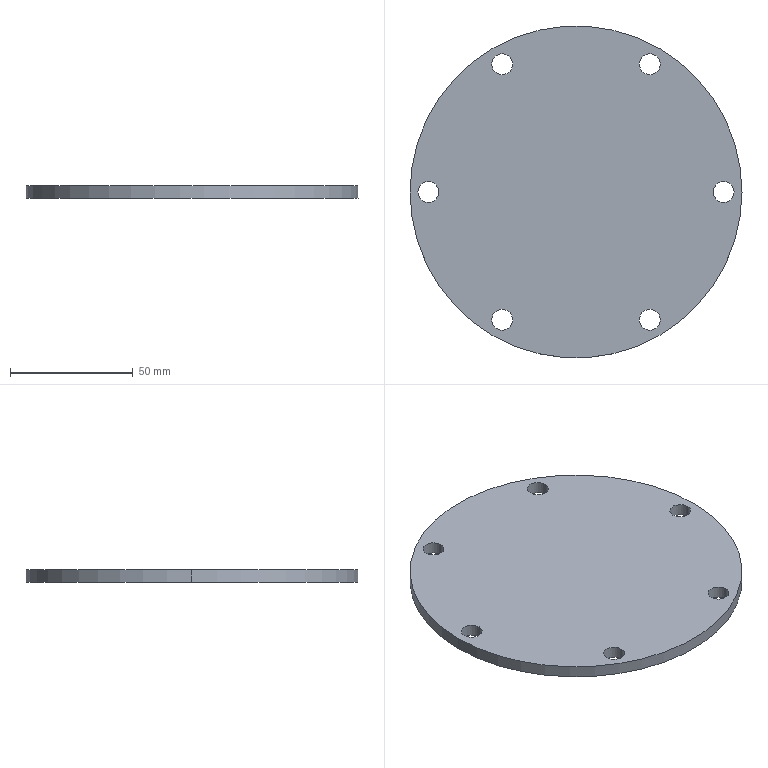Part | SolidWorks | features CirPattern 1, FlatPattern 1, ICE 1, SMBaseFlange 1, SheetMetal 1 | 1 solid | 16 faces | box 135 x 135 x 5 mm | volume 69867 mm3 | cylinder 14 | plane 2 | commonest cylinder face diameters 8.5 x12 135 x2
STEP:
#1=CARTESIAN_POINT('',(25.75,51.962,-5.));
#2=VERTEX_POINT('',#1);
#3=CARTESIAN_POINT('',(34.25,51.962,-5.));
#4=VERTEX_POINT('',#3);
#5=CARTESIAN_POINT('',(30.,51.962,-5.));
#6=DIRECTION('',(0.,0.,1.));
#7=DIRECTION('',(1.,0.,0.));
#8=AXIS2_PLACEMENT_3D('',#5,#6,#7);
#9=CIRCLE('',#8,4.25);
#10=EDGE_CURVE('',#2,#4,#9,.T.);
#11=ORIENTED_EDGE('',*,*,#10,.F.);
#12=CARTESIAN_POINT('',(25.75,51.962,0.));
#13=VERTEX_POINT('',#12);
#14=CARTESIAN_POINT('',(25.75,51.962,-10.));
#15=DIRECTION('',(0.,0.,1.));
#16=VECTOR('',#15,1000.);
#17=LINE('',#14,#16);
#18=EDGE_CURVE('',#2,#13,#17,.T.);
#19=ORIENTED_EDGE('',*,*,#18,.T.);
#20=CARTESIAN_POINT('',(34.25,51.962,0.));
#21=VERTEX_POINT('',#20);
#22=CARTESIAN_POINT('',(30.,51.962,0.));
#23=DIRECTION('',(0.,0.,1.));
#24=DIRECTION('',(0.5,0.866,0.));
#25=AXIS2_PLACEMENT_3D('',#22,#23,#24);
#26=CIRCLE('',#25,4.25);
#27=EDGE_CURVE('',#13,#21,#26,.T.);
#28=ORIENTED_EDGE('',*,*,#27,.T.);
#29=CARTESIAN_POINT('',(34.25,51.962,-10.));
#30=DIRECTION('',(0.,0.,1.));
#31=VECTOR('',#30,1000.);
#32=LINE('',#29,#31);
#33=EDGE_CURVE('',#4,#21,#32,.T.);
#34=ORIENTED_EDGE('',*,*,#33,.F.);
#35=EDGE_LOOP('',(#11,#19,#28,#34));
#36=FACE_OUTER_BOUND('',#35,.T.);
#37=CARTESIAN_POINT('',(30.,51.962,-10.));
#38=DIRECTION('',(0.,0.,1.));
#39=DIRECTION('',(1.,0.,0.));
#40=AXIS2_PLACEMENT_3D('',#37,#38,#39);
#41=CYLINDRICAL_SURFACE('',#40,4.25);
#42=ADVANCED_FACE('',(#36),#41,.F.);
#43=CARTESIAN_POINT('',(-34.25,51.962,-5.));
#44=VERTEX_POINT('',#43);
#45=CARTESIAN_POINT('',(-25.75,51.962,-5.));
#46=VERTEX_POINT('',#45);
#47=CARTESIAN_POINT('',(-30.,51.962,-5.));
#48=DIRECTION('',(0.,0.,1.));
#49=DIRECTION('',(1.,0.,0.));
#50=AXIS2_PLACEMENT_3D('',#47,#48,#49);
#51=CIRCLE('',#50,4.25);
#52=EDGE_CURVE('',#44,#46,#51,.T.);
#53=ORIENTED_EDGE('',*,*,#52,.F.);
#54=CARTESIAN_POINT('',(-34.25,51.962,0.));
#55=VERTEX_POINT('',#54);
#56=CARTESIAN_POINT('',(-34.25,51.962,-10.));
#57=DIRECTION('',(0.,0.,1.));
#58=VECTOR('',#57,1000.);
#59=LINE('',#56,#58);
#60=EDGE_CURVE('',#44,#55,#59,.T.);
#61=ORIENTED_EDGE('',*,*,#60,.T.);
#62=CARTESIAN_POINT('',(-25.75,51.962,0.));
#63=VERTEX_POINT('',#62);
#64=CARTESIAN_POINT('',(-30.,51.962,0.));
#65=DIRECTION('',(0.,0.,1.));
#66=DIRECTION('',(-0.5,0.866,0.));
#67=AXIS2_PLACEMENT_3D('',#64,#65,#66);
#68=CIRCLE('',#67,4.25);
#69=EDGE_CURVE('',#55,#63,#68,.T.);
#70=ORIENTED_EDGE('',*,*,#69,.T.);
#71=CARTESIAN_POINT('',(-25.75,51.962,-10.));
#72=DIRECTION('',(0.,0.,1.));
#73=VECTOR('',#72,1000.);
#74=LINE('',#71,#73);
#75=EDGE_CURVE('',#46,#63,#74,.T.);
#76=ORIENTED_EDGE('',*,*,#75,.F.);
#77=EDGE_LOOP('',(#53,#61,#70,#76));
#78=FACE_OUTER_BOUND('',#77,.T.);
#79=CARTESIAN_POINT('',(-30.,51.962,-10.));
#80=DIRECTION('',(0.,0.,1.));
#81=DIRECTION('',(1.,0.,0.));
#82=AXIS2_PLACEMENT_3D('',#79,#80,#81);
#83=CYLINDRICAL_SURFACE('',#82,4.25);
#84=ADVANCED_FACE('',(#78),#83,.F.);
#85=CARTESIAN_POINT('',(-64.25,0.,-5.));
#86=VERTEX_POINT('',#85);
#87=CARTESIAN_POINT('',(-55.75,0.,-5.));
#88=VERTEX_POINT('',#87);
#89=CARTESIAN_POINT('',(-60.,0.,-5.));
#90=DIRECTION('',(0.,0.,1.));
#91=DIRECTION('',(1.,0.,0.));
#92=AXIS2_PLACEMENT_3D('',#89,#90,#91);
#93=CIRCLE('',#92,4.25);
#94=EDGE_CURVE('',#86,#88,#93,.T.);
#95=ORIENTED_EDGE('',*,*,#94,.F.);
#96=CARTESIAN_POINT('',(-64.25,0.,0.));
#97=VERTEX_POINT('',#96);
#98=CARTESIAN_POINT('',(-64.25,0.,-10.));
#99=DIRECTION('',(0.,0.,1.));
#100=VECTOR('',#99,1000.);
#101=LINE('',#98,#100);
#102=EDGE_CURVE('',#86,#97,#101,.T.);
#103=ORIENTED_EDGE('',*,*,#102,.T.);
#104=CARTESIAN_POINT('',(-55.75,0.,0.));
#105=VERTEX_POINT('',#104);
#106=CARTESIAN_POINT('',(-60.,0.,0.));
#107=DIRECTION('',(0.,0.,1.));
#108=DIRECTION('',(-1.,0.,0.));
#109=AXIS2_PLACEMENT_3D('',#106,#107,#108);
#110=CIRCLE('',#109,4.25);
#111=EDGE_CURVE('',#97,#105,#110,.T.);
#112=ORIENTED_EDGE('',*,*,#111,.T.);
#113=CARTESIAN_POINT('',(-55.75,0.,-10.));
#114=DIRECTION('',(0.,0.,1.));
#115=VECTOR('',#114,1000.);
#116=LINE('',#113,#115);
#117=EDGE_CURVE('',#88,#105,#116,.T.);
#118=ORIENTED_EDGE('',*,*,#117,.F.);
#119=EDGE_LOOP('',(#95,#103,#112,#118));
#120=FACE_OUTER_BOUND('',#119,.T.);
#121=CARTESIAN_POINT('',(-60.,0.,-10.));
#122=DIRECTION('',(0.,0.,1.));
#123=DIRECTION('',(1.,0.,0.));
#124=AXIS2_PLACEMENT_3D('',#121,#122,#123);
#125=CYLINDRICAL_SURFACE('',#124,4.25);
#126=ADVANCED_FACE('',(#120),#125,.F.);
#127=CARTESIAN_POINT('',(-34.25,-51.962,-5.));
#128=VERTEX_POINT('',#127);
#129=CARTESIAN_POINT('',(-25.75,-51.962,-5.));
#130=VERTEX_POINT('',#129);
#131=CARTESIAN_POINT('',(-30.,-51.962,-5.));
#132=DIRECTION('',(0.,0.,1.));
#133=DIRECTION('',(1.,0.,0.));
#134=AXIS2_PLACEMENT_3D('',#131,#132,#133);
#135=CIRCLE('',#134,4.25);
#136=EDGE_CURVE('',#128,#130,#135,.T.);
#137=ORIENTED_EDGE('',*,*,#136,.F.);
#138=CARTESIAN_POINT('',(-34.25,-51.962,0.));
#139=VERTEX_POINT('',#138);
#140=CARTESIAN_POINT('',(-34.25,-51.962,-10.));
#141=DIRECTION('',(0.,0.,1.));
#142=VECTOR('',#141,1000.);
#143=LINE('',#140,#142);
#144=EDGE_CURVE('',#128,#139,#143,.T.);
#145=ORIENTED_EDGE('',*,*,#144,.T.);
#146=CARTESIAN_POINT('',(-25.75,-51.962,0.));
#147=VERTEX_POINT('',#146);
#148=CARTESIAN_POINT('',(-30.,-51.962,0.));
#149=DIRECTION('',(0.,0.,1.));
#150=DIRECTION('',(-0.5,-0.866,0.));
#151=AXIS2_PLACEMENT_3D('',#148,#149,#150);
#152=CIRCLE('',#151,4.25);
#153=EDGE_CURVE('',#139,#147,#152,.T.);
#154=ORIENTED_EDGE('',*,*,#153,.T.);
#155=CARTESIAN_POINT('',(-25.75,-51.962,-10.));
#156=DIRECTION('',(0.,0.,1.));
#157=VECTOR('',#156,1000.);
#158=LINE('',#155,#157);
#159=EDGE_CURVE('',#130,#147,#158,.T.);
#160=ORIENTED_EDGE('',*,*,#159,.F.);
#161=EDGE_LOOP('',(#137,#145,#154,#160));
#162=FACE_OUTER_BOUND('',#161,.T.);
#163=CARTESIAN_POINT('',(-30.,-51.962,-10.));
#164=DIRECTION('',(0.,0.,1.));
#165=DIRECTION('',(1.,0.,0.));
#166=AXIS2_PLACEMENT_3D('',#163,#164,#165);
#167=CYLINDRICAL_SURFACE('',#166,4.25);
#168=ADVANCED_FACE('',(#162),#167,.F.);
#169=CARTESIAN_POINT('',(25.75,-51.962,-5.));
#170=VERTEX_POINT('',#169);
#171=CARTESIAN_POINT('',(34.25,-51.962,-5.));
#172=VERTEX_POINT('',#171);
#173=CARTESIAN_POINT('',(30.,-51.962,-5.));
#174=DIRECTION('',(0.,0.,1.));
#175=DIRECTION('',(1.,0.,0.));
#176=AXIS2_PLACEMENT_3D('',#173,#174,#175);
#177=CIRCLE('',#176,4.25);
#178=EDGE_CURVE('',#170,#172,#177,.T.);
#179=ORIENTED_EDGE('',*,*,#178,.F.);
#180=CARTESIAN_POINT('',(25.75,-51.962,0.));
#181=VERTEX_POINT('',#180);
#182=CARTESIAN_POINT('',(25.75,-51.962,-10.));
#183=DIRECTION('',(0.,0.,1.));
#184=VECTOR('',#183,1000.);
#185=LINE('',#182,#184);
#186=EDGE_CURVE('',#170,#181,#185,.T.);
#187=ORIENTED_EDGE('',*,*,#186,.T.);
#188=CARTESIAN_POINT('',(34.25,-51.962,0.));
#189=VERTEX_POINT('',#188);
#190=CARTESIAN_POINT('',(30.,-51.962,0.));
#191=DIRECTION('',(0.,0.,1.));
#192=DIRECTION('',(0.5,-0.866,0.));
#193=AXIS2_PLACEMENT_3D('',#190,#191,#192);
#194=CIRCLE('',#193,4.25);
#195=EDGE_CURVE('',#181,#189,#194,.T.);
#196=ORIENTED_EDGE('',*,*,#195,.T.);
#197=CARTESIAN_POINT('',(34.25,-51.962,-10.));
#198=DIRECTION('',(0.,0.,1.));
#199=VECTOR('',#198,1000.);
#200=LINE('',#197,#199);
#201=EDGE_CURVE('',#172,#189,#200,.T.);
#202=ORIENTED_EDGE('',*,*,#201,.F.);
#203=EDGE_LOOP('',(#179,#187,#196,#202));
#204=FACE_OUTER_BOUND('',#203,.T.);
#205=CARTESIAN_POINT('',(30.,-51.962,-10.));
#206=DIRECTION('',(0.,0.,1.));
#207=DIRECTION('',(1.,0.,0.));
#208=AXIS2_PLACEMENT_3D('',#205,#206,#207);
#209=CYLINDRICAL_SURFACE('',#208,4.25);
#210=ADVANCED_FACE('',(#204),#209,.F.);
#211=CARTESIAN_POINT('',(55.75,0.,-5.));
#212=VERTEX_POINT('',#211);
#213=CARTESIAN_POINT('',(64.25,0.,-5.));
#214=VERTEX_POINT('',#213);
#215=CARTESIAN_POINT('',(60.,0.,-5.));
#216=DIRECTION('',(0.,0.,1.));
#217=DIRECTION('',(1.,0.,0.));
#218=AXIS2_PLACEMENT_3D('',#215,#216,#217);
#219=CIRCLE('',#218,4.25);
#220=EDGE_CURVE('',#212,#214,#219,.T.);
#221=ORIENTED_EDGE('',*,*,#220,.F.);
#222=CARTESIAN_POINT('',(55.75,0.,0.));
#223=VERTEX_POINT('',#222);
#224=CARTESIAN_POINT('',(55.75,0.,-10.));
#225=DIRECTION('',(0.,0.,1.));
#226=VECTOR('',#225,1000.);
#227=LINE('',#224,#226);
#228=EDGE_CURVE('',#212,#223,#227,.T.);
#229=ORIENTED_EDGE('',*,*,#228,.T.);
#230=CARTESIAN_POINT('',(64.25,0.,0.));
#231=VERTEX_POINT('',#230);
#232=CARTESIAN_POINT('',(60.,0.,0.));
#233=DIRECTION('',(0.,0.,1.));
#234=DIRECTION('',(1.,0.,0.));
#235=AXIS2_PLACEMENT_3D('',#232,#233,#234);
#236=CIRCLE('',#235,4.25);
#237=EDGE_CURVE('',#223,#231,#236,.T.);
#238=ORIENTED_EDGE('',*,*,#237,.T.);
#239=CARTESIAN_POINT('',(64.25,0.,-10.));
#240=DIRECTION('',(0.,0.,1.));
#241=VECTOR('',#240,1000.);
#242=LINE('',#239,#241);
#243=EDGE_CURVE('',#214,#231,#242,.T.);
#244=ORIENTED_EDGE('',*,*,#243,.F.);
#245=EDGE_LOOP('',(#221,#229,#238,#244));
#246=FACE_OUTER_BOUND('',#245,.T.);
#247=CARTESIAN_POINT('',(60.,0.,-10.));
#248=DIRECTION('',(0.,0.,1.));
#249=DIRECTION('',(1.,0.,0.));
#250=AXIS2_PLACEMENT_3D('',#247,#248,#249);
#251=CYLINDRICAL_SURFACE('',#250,4.25);
#252=ADVANCED_FACE('',(#246),#251,.F.);
#253=CARTESIAN_POINT('',(67.5,0.,-5.));
#254=VERTEX_POINT('',#253);
#255=CARTESIAN_POINT('',(-67.5,0.,-5.));
#256=VERTEX_POINT('',#255);
#257=CARTESIAN_POINT('',(0.,0.,-5.));
#258=DIRECTION('',(0.,0.,1.));
#259=DIRECTION('',(1.,0.,0.));
#260=AXIS2_PLACEMENT_3D('',#257,#258,#259);
#261=CIRCLE('',#260,67.5);
#262=EDGE_CURVE('',#254,#256,#261,.T.);
#263=ORIENTED_EDGE('',*,*,#262,.T.);
#264=CARTESIAN_POINT('',(-67.5,0.,0.));
#265=VERTEX_POINT('',#264);
#266=CARTESIAN_POINT('',(-67.5,0.,-5.));
#267=DIRECTION('',(0.,0.,1.));
#268=VECTOR('',#267,1000.);
#269=LINE('',#266,#268);
#270=EDGE_CURVE('',#256,#265,#269,.T.);
#271=ORIENTED_EDGE('',*,*,#270,.T.);
#272=CARTESIAN_POINT('',(67.5,0.,0.));
#273=VERTEX_POINT('',#272);
#274=CARTESIAN_POINT('',(0.,0.,0.));
#275=DIRECTION('',(0.,0.,1.));
#276=DIRECTION('',(1.,0.,0.));
#277=AXIS2_PLACEMENT_3D('',#274,#275,#276);
#278=CIRCLE('',#277,67.5);
#279=EDGE_CURVE('',#273,#265,#278,.T.);
#280=ORIENTED_EDGE('',*,*,#279,.F.);
#281=CARTESIAN_POINT('',(67.5,0.,-5.));
#282=DIRECTION('',(0.,0.,1.));
#283=VECTOR('',#282,1000.);
#284=LINE('',#281,#283);
#285=EDGE_CURVE('',#254,#273,#284,.T.);
#286=ORIENTED_EDGE('',*,*,#285,.F.);
#287=EDGE_LOOP('',(#263,#271,#280,#286));
#288=FACE_OUTER_BOUND('',#287,.T.);
#289=CARTESIAN_POINT('',(0.,0.,-5.));
#290=DIRECTION('',(0.,0.,1.));
#291=DIRECTION('',(1.,0.,0.));
#292=AXIS2_PLACEMENT_3D('',#289,#290,#291);
#293=CYLINDRICAL_SURFACE('',#292,67.5);
#294=ADVANCED_FACE('',(#288),#293,.T.);
#295=ORIENTED_EDGE('',*,*,#270,.F.);
#296=CARTESIAN_POINT('',(0.,0.,-5.));
#297=DIRECTION('',(0.,0.,1.));
#298=DIRECTION('',(1.,0.,0.));
#299=AXIS2_PLACEMENT_3D('',#296,#297,#298);
#300=CIRCLE('',#299,67.5);
#301=EDGE_CURVE('',#256,#254,#300,.T.);
#302=ORIENTED_EDGE('',*,*,#301,.T.);
#303=ORIENTED_EDGE('',*,*,#285,.T.);
#304=CARTESIAN_POINT('',(0.,0.,0.));
#305=DIRECTION('',(0.,0.,1.));
#306=DIRECTION('',(1.,0.,0.));
#307=AXIS2_PLACEMENT_3D('',#304,#305,#306);
#308=CIRCLE('',#307,67.5);
#309=EDGE_CURVE('',#265,#273,#308,.T.);
#310=ORIENTED_EDGE('',*,*,#309,.F.);
#311=EDGE_LOOP('',(#295,#302,#303,#310));
#312=FACE_OUTER_BOUND('',#311,.T.);
#313=CARTESIAN_POINT('',(0.,0.,-5.));
#314=DIRECTION('',(0.,0.,1.));
#315=DIRECTION('',(1.,0.,0.));
#316=AXIS2_PLACEMENT_3D('',#313,#314,#315);
#317=CYLINDRICAL_SURFACE('',#316,67.5);
#318=ADVANCED_FACE('',(#312),#317,.T.);
#319=CARTESIAN_POINT('',(30.,51.962,-5.));
#320=DIRECTION('',(0.,0.,1.));
#321=DIRECTION('',(1.,0.,0.));
#322=AXIS2_PLACEMENT_3D('',#319,#320,#321);
#323=CIRCLE('',#322,4.25);
#324=EDGE_CURVE('',#4,#2,#323,.T.);
#325=ORIENTED_EDGE('',*,*,#324,.T.);
#326=ORIENTED_EDGE('',*,*,#10,.T.);
#327=EDGE_LOOP('',(#325,#326));
#328=FACE_BOUND('',#327,.T.);
#329=CARTESIAN_POINT('',(-30.,51.962,-5.));
#330=DIRECTION('',(0.,0.,1.));
#331=DIRECTION('',(1.,0.,0.));
#332=AXIS2_PLACEMENT_3D('',#329,#330,#331);
#333=CIRCLE('',#332,4.25);
#334=EDGE_CURVE('',#46,#44,#333,.T.);
#335=ORIENTED_EDGE('',*,*,#334,.T.);
#336=ORIENTED_EDGE('',*,*,#52,.T.);
#337=EDGE_LOOP('',(#335,#336));
#338=FACE_BOUND('',#337,.T.);
#339=CARTESIAN_POINT('',(-60.,0.,-5.));
#340=DIRECTION('',(0.,0.,1.));
#341=DIRECTION('',(1.,0.,0.));
#342=AXIS2_PLACEMENT_3D('',#339,#340,#341);
#343=CIRCLE('',#342,4.25);
#344=EDGE_CURVE('',#88,#86,#343,.T.);
#345=ORIENTED_EDGE('',*,*,#344,.T.);
#346=ORIENTED_EDGE('',*,*,#94,.T.);
#347=EDGE_LOOP('',(#345,#346));
#348=FACE_BOUND('',#347,.T.);
#349=CARTESIAN_POINT('',(-30.,-51.962,-5.));
#350=DIRECTION('',(0.,0.,1.));
#351=DIRECTION('',(1.,0.,0.));
#352=AXIS2_PLACEMENT_3D('',#349,#350,#351);
#353=CIRCLE('',#352,4.25);
#354=EDGE_CURVE('',#130,#128,#353,.T.);
#355=ORIENTED_EDGE('',*,*,#354,.T.);
#356=ORIENTED_EDGE('',*,*,#136,.T.);
#357=EDGE_LOOP('',(#355,#356));
#358=FACE_BOUND('',#357,.T.);
#359=CARTESIAN_POINT('',(30.,-51.962,-5.));
#360=DIRECTION('',(0.,0.,1.));
#361=DIRECTION('',(1.,0.,0.));
#362=AXIS2_PLACEMENT_3D('',#359,#360,#361);
#363=CIRCLE('',#362,4.25);
#364=EDGE_CURVE('',#172,#170,#363,.T.);
#365=ORIENTED_EDGE('',*,*,#364,.T.);
#366=ORIENTED_EDGE('',*,*,#178,.T.);
#367=EDGE_LOOP('',(#365,#366));
#368=FACE_BOUND('',#367,.T.);
#369=CARTESIAN_POINT('',(60.,0.,-5.));
#370=DIRECTION('',(0.,0.,1.));
#371=DIRECTION('',(1.,0.,0.));
#372=AXIS2_PLACEMENT_3D('',#369,#370,#371);
#373=CIRCLE('',#372,4.25);
#374=EDGE_CURVE('',#214,#212,#373,.T.);
#375=ORIENTED_EDGE('',*,*,#374,.T.);
#376=ORIENTED_EDGE('',*,*,#220,.T.);
#377=EDGE_LOOP('',(#375,#376));
#378=FACE_BOUND('',#377,.T.);
#379=ORIENTED_EDGE('',*,*,#262,.F.);
#380=ORIENTED_EDGE('',*,*,#301,.F.);
#381=EDGE_LOOP('',(#379,#380));
#382=FACE_OUTER_BOUND('',#381,.T.);
#383=CARTESIAN_POINT('',(0.,0.,-5.));
#384=DIRECTION('',(0.,0.,1.));
#385=DIRECTION('',(1.,0.,0.));
#386=AXIS2_PLACEMENT_3D('',#383,#384,#385);
#387=PLANE('',#386);
#388=ADVANCED_FACE('',(#328,#338,#348,#358,#368,#378,#382),#387,.F.);
#389=CARTESIAN_POINT('',(30.,51.962,0.));
#390=DIRECTION('',(0.,0.,1.));
#391=DIRECTION('',(0.5,0.866,0.));
#392=AXIS2_PLACEMENT_3D('',#389,#390,#391);
#393=CIRCLE('',#392,4.25);
#394=EDGE_CURVE('',#21,#13,#393,.T.);
#395=ORIENTED_EDGE('',*,*,#394,.F.);
#396=ORIENTED_EDGE('',*,*,#27,.F.);
#397=EDGE_LOOP('',(#395,#396));
#398=FACE_BOUND('',#397,.T.);
#399=CARTESIAN_POINT('',(-30.,51.962,0.));
#400=DIRECTION('',(0.,0.,1.));
#401=DIRECTION('',(-0.5,0.866,0.));
#402=AXIS2_PLACEMENT_3D('',#399,#400,#401);
#403=CIRCLE('',#402,4.25);
#404=EDGE_CURVE('',#63,#55,#403,.T.);
#405=ORIENTED_EDGE('',*,*,#404,.F.);
#406=ORIENTED_EDGE('',*,*,#69,.F.);
#407=EDGE_LOOP('',(#405,#406));
#408=FACE_BOUND('',#407,.T.);
#409=CARTESIAN_POINT('',(-60.,0.,0.));
#410=DIRECTION('',(0.,0.,1.));
#411=DIRECTION('',(-1.,0.,0.));
#412=AXIS2_PLACEMENT_3D('',#409,#410,#411);
#413=CIRCLE('',#412,4.25);
#414=EDGE_CURVE('',#105,#97,#413,.T.);
#415=ORIENTED_EDGE('',*,*,#414,.F.);
#416=ORIENTED_EDGE('',*,*,#111,.F.);
#417=EDGE_LOOP('',(#415,#416));
#418=FACE_BOUND('',#417,.T.);
#419=CARTESIAN_POINT('',(-30.,-51.962,0.));
#420=DIRECTION('',(0.,0.,1.));
#421=DIRECTION('',(-0.5,-0.866,0.));
#422=AXIS2_PLACEMENT_3D('',#419,#420,#421);
#423=CIRCLE('',#422,4.25);
#424=EDGE_CURVE('',#147,#139,#423,.T.);
#425=ORIENTED_EDGE('',*,*,#424,.F.);
#426=ORIENTED_EDGE('',*,*,#153,.F.);
#427=EDGE_LOOP('',(#425,#426));
#428=FACE_BOUND('',#427,.T.);
#429=CARTESIAN_POINT('',(30.,-51.962,0.));
#430=DIRECTION('',(0.,0.,1.));
#431=DIRECTION('',(0.5,-0.866,0.));
#432=AXIS2_PLACEMENT_3D('',#429,#430,#431);
#433=CIRCLE('',#432,4.25);
#434=EDGE_CURVE('',#189,#181,#433,.T.);
#435=ORIENTED_EDGE('',*,*,#434,.F.);
#436=ORIENTED_EDGE('',*,*,#195,.F.);
#437=EDGE_LOOP('',(#435,#436));
#438=FACE_BOUND('',#437,.T.);
#439=CARTESIAN_POINT('',(60.,0.,0.));
#440=DIRECTION('',(0.,0.,1.));
#441=DIRECTION('',(1.,0.,0.));
#442=AXIS2_PLACEMENT_3D('',#439,#440,#441);
#443=CIRCLE('',#442,4.25);
#444=EDGE_CURVE('',#231,#223,#443,.T.);
#445=ORIENTED_EDGE('',*,*,#444,.F.);
#446=ORIENTED_EDGE('',*,*,#237,.F.);
#447=EDGE_LOOP('',(#445,#446));
#448=FACE_BOUND('',#447,.T.);
#449=ORIENTED_EDGE('',*,*,#279,.T.);
#450=ORIENTED_EDGE('',*,*,#309,.T.);
#451=EDGE_LOOP('',(#449,#450));
#452=FACE_OUTER_BOUND('',#451,.T.);
#453=CARTESIAN_POINT('',(0.,0.,0.));
#454=DIRECTION('',(0.,0.,1.));
#455=DIRECTION('',(1.,0.,0.));
#456=AXIS2_PLACEMENT_3D('',#453,#454,#455);
#457=PLANE('',#456);
#458=ADVANCED_FACE('',(#398,#408,#418,#428,#438,#448,#452),#457,.T.);
#459=ORIENTED_EDGE('',*,*,#228,.F.);
#460=ORIENTED_EDGE('',*,*,#374,.F.);
#461=ORIENTED_EDGE('',*,*,#243,.T.);
#462=ORIENTED_EDGE('',*,*,#444,.T.);
#463=EDGE_LOOP('',(#459,#460,#461,#462));
#464=FACE_OUTER_BOUND('',#463,.T.);
#465=CARTESIAN_POINT('',(60.,0.,-10.));
#466=DIRECTION('',(0.,0.,1.));
#467=DIRECTION('',(1.,0.,0.));
#468=AXIS2_PLACEMENT_3D('',#465,#466,#467);
#469=CYLINDRICAL_SURFACE('',#468,4.25);
#470=ADVANCED_FACE('',(#464),#469,.F.);
#471=ORIENTED_EDGE('',*,*,#186,.F.);
#472=ORIENTED_EDGE('',*,*,#364,.F.);
#473=ORIENTED_EDGE('',*,*,#201,.T.);
#474=ORIENTED_EDGE('',*,*,#434,.T.);
#475=EDGE_LOOP('',(#471,#472,#473,#474));
#476=FACE_OUTER_BOUND('',#475,.T.);
#477=CARTESIAN_POINT('',(30.,-51.962,-10.));
#478=DIRECTION('',(0.,0.,1.));
#479=DIRECTION('',(1.,0.,0.));
#480=AXIS2_PLACEMENT_3D('',#477,#478,#479);
#481=CYLINDRICAL_SURFACE('',#480,4.25);
#482=ADVANCED_FACE('',(#476),#481,.F.);
#483=ORIENTED_EDGE('',*,*,#144,.F.);
#484=ORIENTED_EDGE('',*,*,#354,.F.);
#485=ORIENTED_EDGE('',*,*,#159,.T.);
#486=ORIENTED_EDGE('',*,*,#424,.T.);
#487=EDGE_LOOP('',(#483,#484,#485,#486));
#488=FACE_OUTER_BOUND('',#487,.T.);
#489=CARTESIAN_POINT('',(-30.,-51.962,-10.));
#490=DIRECTION('',(0.,0.,1.));
#491=DIRECTION('',(1.,0.,0.));
#492=AXIS2_PLACEMENT_3D('',#489,#490,#491);
#493=CYLINDRICAL_SURFACE('',#492,4.25);
#494=ADVANCED_FACE('',(#488),#493,.F.);
#495=ORIENTED_EDGE('',*,*,#102,.F.);
#496=ORIENTED_EDGE('',*,*,#344,.F.);
#497=ORIENTED_EDGE('',*,*,#117,.T.);
#498=ORIENTED_EDGE('',*,*,#414,.T.);
#499=EDGE_LOOP('',(#495,#496,#497,#498));
#500=FACE_OUTER_BOUND('',#499,.T.);
#501=CARTESIAN_POINT('',(-60.,0.,-10.));
#502=DIRECTION('',(0.,0.,1.));
#503=DIRECTION('',(1.,0.,0.));
#504=AXIS2_PLACEMENT_3D('',#501,#502,#503);
#505=CYLINDRICAL_SURFACE('',#504,4.25);
#506=ADVANCED_FACE('',(#500),#505,.F.);
#507=ORIENTED_EDGE('',*,*,#60,.F.);
#508=ORIENTED_EDGE('',*,*,#334,.F.);
#509=ORIENTED_EDGE('',*,*,#75,.T.);
#510=ORIENTED_EDGE('',*,*,#404,.T.);
#511=EDGE_LOOP('',(#507,#508,#509,#510));
#512=FACE_OUTER_BOUND('',#511,.T.);
#513=CARTESIAN_POINT('',(-30.,51.962,-10.));
#514=DIRECTION('',(0.,0.,1.));
#515=DIRECTION('',(1.,0.,0.));
#516=AXIS2_PLACEMENT_3D('',#513,#514,#515);
#517=CYLINDRICAL_SURFACE('',#516,4.25);
#518=ADVANCED_FACE('',(#512),#517,.F.);
#519=ORIENTED_EDGE('',*,*,#18,.F.);
#520=ORIENTED_EDGE('',*,*,#324,.F.);
#521=ORIENTED_EDGE('',*,*,#33,.T.);
#522=ORIENTED_EDGE('',*,*,#394,.T.);
#523=EDGE_LOOP('',(#519,#520,#521,#522));
#524=FACE_OUTER_BOUND('',#523,.T.);
#525=CARTESIAN_POINT('',(30.,51.962,-10.));
#526=DIRECTION('',(0.,0.,1.));
#527=DIRECTION('',(1.,0.,0.));
#528=AXIS2_PLACEMENT_3D('',#525,#526,#527);
#529=CYLINDRICAL_SURFACE('',#528,4.25);
#530=ADVANCED_FACE('',(#524),#529,.F.);
#531=CLOSED_SHELL('',(#42,#84,#126,#168,#210,#252,#294,#318,#388,#458,#470,#482,#494,#506,#518,#530));
#532=MANIFOLD_SOLID_BREP('',#531);
#533=CARTESIAN_POINT('',(0.,0.,0.));
#534=DIRECTION('',(0.,0.,1.));
#535=DIRECTION('',(1.,0.,0.));
#536=AXIS2_PLACEMENT_3D('',#533,#534,#535);
#537=(LENGTH_UNIT()NAMED_UNIT(*)SI_UNIT(.MILLI.,.METRE.));
#538=UNCERTAINTY_MEASURE_WITH_UNIT(LENGTH_MEASURE(0.00001),#537,'','');
#539=(NAMED_UNIT(*)PLANE_ANGLE_UNIT()SI_UNIT($,.RADIAN.));
#540=(NAMED_UNIT(*)SI_UNIT($,.STERADIAN.)SOLID_ANGLE_UNIT());
#541=(GEOMETRIC_REPRESENTATION_CONTEXT(3)GLOBAL_UNCERTAINTY_ASSIGNED_CONTEXT((#538))GLOBAL_UNIT_ASSIGNED_CONTEXT((#537,#539,#540))REPRESENTATION_CONTEXT('',''));
#542=ADVANCED_BREP_SHAPE_REPRESENTATION('',(#532,#536),#541);